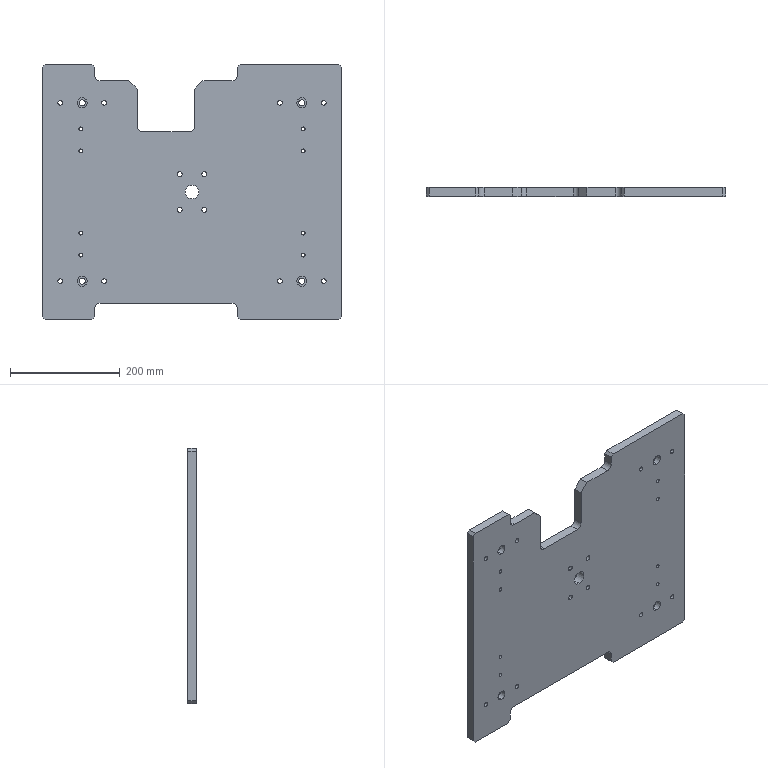Part | SolidWorks | features HoleWzd 5, MirrorPattern 5, ICE 4, Chamfer 2, Extrusion 1, Fillet 1 | 1 solid | 96 faces | box 545 x 16 x 465 mm | volume 3609981 mm3 | cylinder 64 | plane 32 | commonest cylinder face diameters 6.8 x16 8.5 x16 9 x8 11 x8 18 x8 20 x6